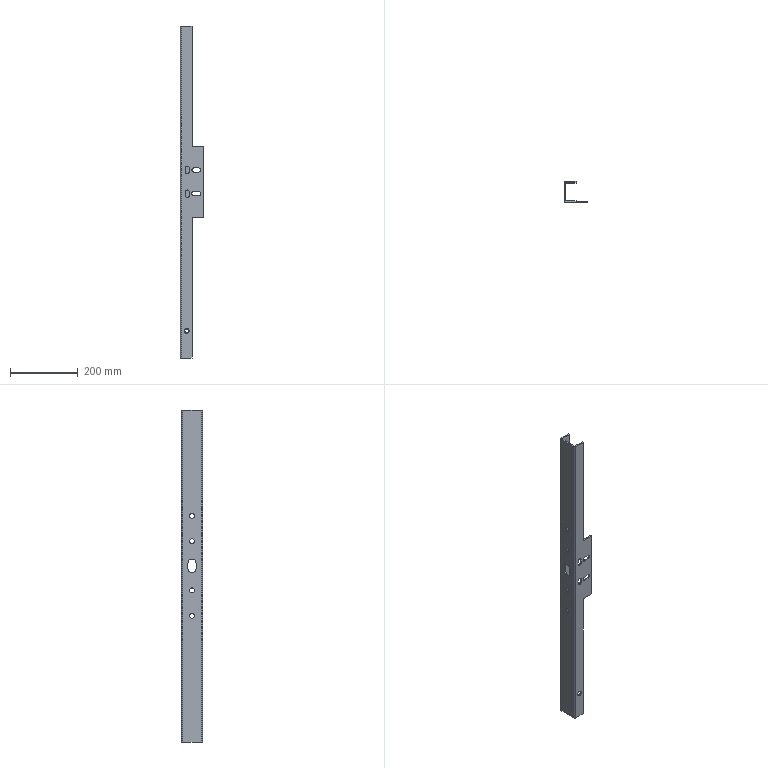Part | 1 solid | 82 faces | box 70 x 62 x 980 mm | volume 491604 mm3 | plane 42 | cylinder 40 | commonest cylinder face diameters 10 x12 12 x10 14.5 x8 0.4 x2 8.4 x2 11 x2